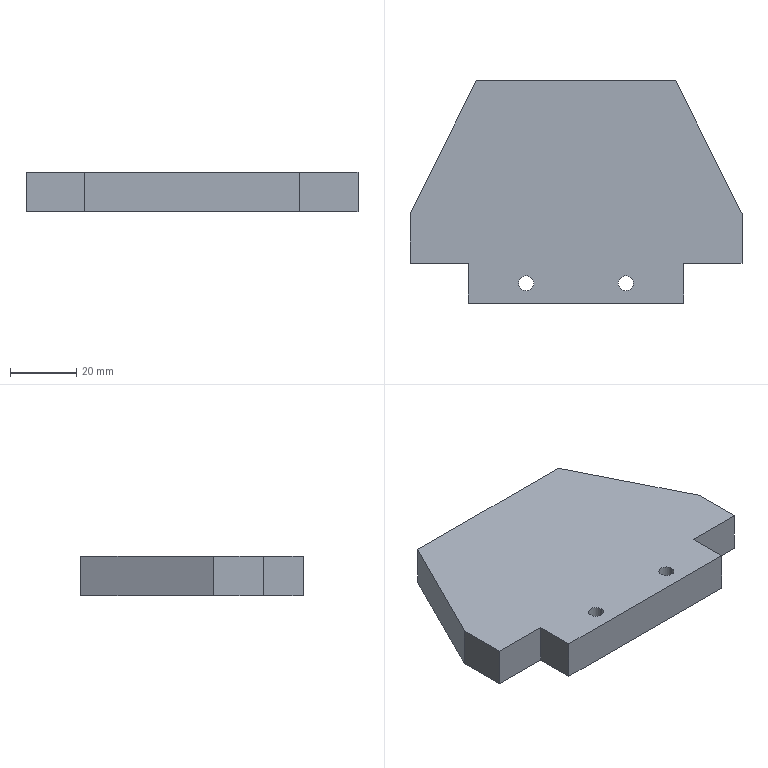Part | SolidWorks | features Chamfer 2, Extrusion 1, HoleWzd 1, ICE 1 | 1 solid | 22 faces | box 100 x 67 x 12 mm | volume 65076 mm3 | plane 14 | cylinder 8 | commonest cylinder face diameters 4.5 x4 8 x4
STEP:
#1=CARTESIAN_POINT('',(-11.,-33.5,4.4));
#2=VERTEX_POINT('',#1);
#3=CARTESIAN_POINT('',(-19.,-33.5,4.4));
#4=VERTEX_POINT('',#3);
#5=CARTESIAN_POINT('',(-15.,-33.5,4.4));
#6=DIRECTION('',(0.,0.,-1.));
#7=DIRECTION('',(-1.,0.,0.));
#8=AXIS2_PLACEMENT_3D('',#5,#6,#7);
#9=CIRCLE('',#8,4.);
#10=EDGE_CURVE('',#2,#4,#9,.T.);
#11=ORIENTED_EDGE('',*,*,#10,.F.);
#12=CARTESIAN_POINT('',(-11.,-33.5,0.));
#13=VERTEX_POINT('',#12);
#14=CARTESIAN_POINT('',(-11.,-33.5,0.));
#15=DIRECTION('',(0.,0.,-1.));
#16=VECTOR('',#15,1000.);
#17=LINE('',#14,#16);
#18=EDGE_CURVE('',#2,#13,#17,.T.);
#19=ORIENTED_EDGE('',*,*,#18,.T.);
#20=CARTESIAN_POINT('',(-19.,-33.5,0.));
#21=VERTEX_POINT('',#20);
#22=CARTESIAN_POINT('',(-15.,-33.5,0.));
#23=DIRECTION('',(0.,0.,-1.));
#24=DIRECTION('',(-1.,0.,0.));
#25=AXIS2_PLACEMENT_3D('',#22,#23,#24);
#26=CIRCLE('',#25,4.);
#27=EDGE_CURVE('',#13,#21,#26,.T.);
#28=ORIENTED_EDGE('',*,*,#27,.T.);
#29=CARTESIAN_POINT('',(-19.,-33.5,0.));
#30=DIRECTION('',(0.,0.,-1.));
#31=VECTOR('',#30,1000.);
#32=LINE('',#29,#31);
#33=EDGE_CURVE('',#4,#21,#32,.T.);
#34=ORIENTED_EDGE('',*,*,#33,.F.);
#35=EDGE_LOOP('',(#11,#19,#28,#34));
#36=FACE_OUTER_BOUND('',#35,.T.);
#37=CARTESIAN_POINT('',(-15.,-33.5,0.));
#38=DIRECTION('',(0.,0.,-1.));
#39=DIRECTION('',(-1.,0.,0.));
#40=AXIS2_PLACEMENT_3D('',#37,#38,#39);
#41=CYLINDRICAL_SURFACE('',#40,4.);
#42=ADVANCED_FACE('',(#36),#41,.F.);
#43=CARTESIAN_POINT('',(-12.75,-33.5,12.));
#44=VERTEX_POINT('',#43);
#45=CARTESIAN_POINT('',(-17.25,-33.5,12.));
#46=VERTEX_POINT('',#45);
#47=CARTESIAN_POINT('',(-15.,-33.5,12.));
#48=DIRECTION('',(0.,0.,-1.));
#49=DIRECTION('',(-1.,0.,0.));
#50=AXIS2_PLACEMENT_3D('',#47,#48,#49);
#51=CIRCLE('',#50,2.25);
#52=EDGE_CURVE('',#44,#46,#51,.T.);
#53=ORIENTED_EDGE('',*,*,#52,.F.);
#54=CARTESIAN_POINT('',(-12.75,-33.5,4.4));
#55=VERTEX_POINT('',#54);
#56=CARTESIAN_POINT('',(-12.75,-33.5,0.));
#57=DIRECTION('',(0.,0.,-1.));
#58=VECTOR('',#57,1000.);
#59=LINE('',#56,#58);
#60=EDGE_CURVE('',#44,#55,#59,.T.);
#61=ORIENTED_EDGE('',*,*,#60,.T.);
#62=CARTESIAN_POINT('',(-17.25,-33.5,4.4));
#63=VERTEX_POINT('',#62);
#64=CARTESIAN_POINT('',(-15.,-33.5,4.4));
#65=DIRECTION('',(0.,0.,-1.));
#66=DIRECTION('',(-1.,0.,0.));
#67=AXIS2_PLACEMENT_3D('',#64,#65,#66);
#68=CIRCLE('',#67,2.25);
#69=EDGE_CURVE('',#55,#63,#68,.T.);
#70=ORIENTED_EDGE('',*,*,#69,.T.);
#71=CARTESIAN_POINT('',(-17.25,-33.5,0.));
#72=DIRECTION('',(0.,0.,-1.));
#73=VECTOR('',#72,1000.);
#74=LINE('',#71,#73);
#75=EDGE_CURVE('',#46,#63,#74,.T.);
#76=ORIENTED_EDGE('',*,*,#75,.F.);
#77=EDGE_LOOP('',(#53,#61,#70,#76));
#78=FACE_OUTER_BOUND('',#77,.T.);
#79=CARTESIAN_POINT('',(-15.,-33.5,0.));
#80=DIRECTION('',(0.,0.,-1.));
#81=DIRECTION('',(-1.,0.,0.));
#82=AXIS2_PLACEMENT_3D('',#79,#80,#81);
#83=CYLINDRICAL_SURFACE('',#82,2.25);
#84=ADVANCED_FACE('',(#78),#83,.F.);
#85=CARTESIAN_POINT('',(19.,-33.5,4.4));
#86=VERTEX_POINT('',#85);
#87=CARTESIAN_POINT('',(11.,-33.5,4.4));
#88=VERTEX_POINT('',#87);
#89=CARTESIAN_POINT('',(15.,-33.5,4.4));
#90=DIRECTION('',(0.,0.,-1.));
#91=DIRECTION('',(-1.,0.,0.));
#92=AXIS2_PLACEMENT_3D('',#89,#90,#91);
#93=CIRCLE('',#92,4.);
#94=EDGE_CURVE('',#86,#88,#93,.T.);
#95=ORIENTED_EDGE('',*,*,#94,.F.);
#96=CARTESIAN_POINT('',(19.,-33.5,0.));
#97=VERTEX_POINT('',#96);
#98=CARTESIAN_POINT('',(19.,-33.5,0.));
#99=DIRECTION('',(0.,0.,-1.));
#100=VECTOR('',#99,1000.);
#101=LINE('',#98,#100);
#102=EDGE_CURVE('',#86,#97,#101,.T.);
#103=ORIENTED_EDGE('',*,*,#102,.T.);
#104=CARTESIAN_POINT('',(11.,-33.5,0.));
#105=VERTEX_POINT('',#104);
#106=CARTESIAN_POINT('',(15.,-33.5,0.));
#107=DIRECTION('',(0.,0.,-1.));
#108=DIRECTION('',(-1.,0.,0.));
#109=AXIS2_PLACEMENT_3D('',#106,#107,#108);
#110=CIRCLE('',#109,4.);
#111=EDGE_CURVE('',#97,#105,#110,.T.);
#112=ORIENTED_EDGE('',*,*,#111,.T.);
#113=CARTESIAN_POINT('',(11.,-33.5,0.));
#114=DIRECTION('',(0.,0.,-1.));
#115=VECTOR('',#114,1000.);
#116=LINE('',#113,#115);
#117=EDGE_CURVE('',#88,#105,#116,.T.);
#118=ORIENTED_EDGE('',*,*,#117,.F.);
#119=EDGE_LOOP('',(#95,#103,#112,#118));
#120=FACE_OUTER_BOUND('',#119,.T.);
#121=CARTESIAN_POINT('',(15.,-33.5,0.));
#122=DIRECTION('',(0.,0.,-1.));
#123=DIRECTION('',(-1.,0.,0.));
#124=AXIS2_PLACEMENT_3D('',#121,#122,#123);
#125=CYLINDRICAL_SURFACE('',#124,4.);
#126=ADVANCED_FACE('',(#120),#125,.F.);
#127=CARTESIAN_POINT('',(17.25,-33.5,12.));
#128=VERTEX_POINT('',#127);
#129=CARTESIAN_POINT('',(12.75,-33.5,12.));
#130=VERTEX_POINT('',#129);
#131=CARTESIAN_POINT('',(15.,-33.5,12.));
#132=DIRECTION('',(0.,0.,-1.));
#133=DIRECTION('',(-1.,0.,0.));
#134=AXIS2_PLACEMENT_3D('',#131,#132,#133);
#135=CIRCLE('',#134,2.25);
#136=EDGE_CURVE('',#128,#130,#135,.T.);
#137=ORIENTED_EDGE('',*,*,#136,.F.);
#138=CARTESIAN_POINT('',(17.25,-33.5,4.4));
#139=VERTEX_POINT('',#138);
#140=CARTESIAN_POINT('',(17.25,-33.5,0.));
#141=DIRECTION('',(0.,0.,-1.));
#142=VECTOR('',#141,1000.);
#143=LINE('',#140,#142);
#144=EDGE_CURVE('',#128,#139,#143,.T.);
#145=ORIENTED_EDGE('',*,*,#144,.T.);
#146=CARTESIAN_POINT('',(12.75,-33.5,4.4));
#147=VERTEX_POINT('',#146);
#148=CARTESIAN_POINT('',(15.,-33.5,4.4));
#149=DIRECTION('',(0.,0.,-1.));
#150=DIRECTION('',(-1.,0.,0.));
#151=AXIS2_PLACEMENT_3D('',#148,#149,#150);
#152=CIRCLE('',#151,2.25);
#153=EDGE_CURVE('',#139,#147,#152,.T.);
#154=ORIENTED_EDGE('',*,*,#153,.T.);
#155=CARTESIAN_POINT('',(12.75,-33.5,0.));
#156=DIRECTION('',(0.,0.,-1.));
#157=VECTOR('',#156,1000.);
#158=LINE('',#155,#157);
#159=EDGE_CURVE('',#130,#147,#158,.T.);
#160=ORIENTED_EDGE('',*,*,#159,.F.);
#161=EDGE_LOOP('',(#137,#145,#154,#160));
#162=FACE_OUTER_BOUND('',#161,.T.);
#163=CARTESIAN_POINT('',(15.,-33.5,0.));
#164=DIRECTION('',(0.,0.,-1.));
#165=DIRECTION('',(-1.,0.,0.));
#166=AXIS2_PLACEMENT_3D('',#163,#164,#165);
#167=CYLINDRICAL_SURFACE('',#166,2.25);
#168=ADVANCED_FACE('',(#162),#167,.F.);
#169=CARTESIAN_POINT('',(-32.5,-27.5,12.));
#170=VERTEX_POINT('',#169);
#171=CARTESIAN_POINT('',(-32.5,-27.5,0.));
#172=VERTEX_POINT('',#171);
#173=CARTESIAN_POINT('',(-32.5,-27.5,12.));
#174=DIRECTION('',(0.,0.,-1.));
#175=VECTOR('',#174,1000.);
#176=LINE('',#173,#175);
#177=EDGE_CURVE('',#170,#172,#176,.T.);
#178=ORIENTED_EDGE('',*,*,#177,.F.);
#179=CARTESIAN_POINT('',(-50.,-27.5,12.));
#180=VERTEX_POINT('',#179);
#181=CARTESIAN_POINT('',(-50.,-27.5,12.));
#182=DIRECTION('',(1.,0.,0.));
#183=VECTOR('',#182,1000.);
#184=LINE('',#181,#183);
#185=EDGE_CURVE('',#180,#170,#184,.T.);
#186=ORIENTED_EDGE('',*,*,#185,.F.);
#187=CARTESIAN_POINT('',(-50.,-27.5,0.));
#188=VERTEX_POINT('',#187);
#189=CARTESIAN_POINT('',(-50.,-27.5,12.));
#190=DIRECTION('',(0.,0.,-1.));
#191=VECTOR('',#190,1000.);
#192=LINE('',#189,#191);
#193=EDGE_CURVE('',#180,#188,#192,.T.);
#194=ORIENTED_EDGE('',*,*,#193,.T.);
#195=CARTESIAN_POINT('',(-50.,-27.5,0.));
#196=DIRECTION('',(1.,0.,0.));
#197=VECTOR('',#196,1000.);
#198=LINE('',#195,#197);
#199=EDGE_CURVE('',#188,#172,#198,.T.);
#200=ORIENTED_EDGE('',*,*,#199,.T.);
#201=EDGE_LOOP('',(#178,#186,#194,#200));
#202=FACE_OUTER_BOUND('',#201,.T.);
#203=CARTESIAN_POINT('',(-50.,-27.5,12.));
#204=DIRECTION('',(0.,1.,0.));
#205=DIRECTION('',(0.,0.,1.));
#206=AXIS2_PLACEMENT_3D('',#203,#204,#205);
#207=PLANE('',#206);
#208=ADVANCED_FACE('',(#202),#207,.F.);
#209=CARTESIAN_POINT('',(32.5,-27.5,0.));
#210=VERTEX_POINT('',#209);
#211=CARTESIAN_POINT('',(32.5,-27.5,12.));
#212=VERTEX_POINT('',#211);
#213=CARTESIAN_POINT('',(32.5,-27.5,12.));
#214=DIRECTION('',(0.,0.,1.));
#215=VECTOR('',#214,1000.);
#216=LINE('',#213,#215);
#217=EDGE_CURVE('',#210,#212,#216,.T.);
#218=ORIENTED_EDGE('',*,*,#217,.F.);
#219=CARTESIAN_POINT('',(50.,-27.5,0.));
#220=VERTEX_POINT('',#219);
#221=CARTESIAN_POINT('',(-50.,-27.5,0.));
#222=DIRECTION('',(1.,0.,0.));
#223=VECTOR('',#222,1000.);
#224=LINE('',#221,#223);
#225=EDGE_CURVE('',#210,#220,#224,.T.);
#226=ORIENTED_EDGE('',*,*,#225,.T.);
#227=CARTESIAN_POINT('',(50.,-27.5,12.));
#228=VERTEX_POINT('',#227);
#229=CARTESIAN_POINT('',(50.,-27.5,12.));
#230=DIRECTION('',(0.,0.,-1.));
#231=VECTOR('',#230,1000.);
#232=LINE('',#229,#231);
#233=EDGE_CURVE('',#228,#220,#232,.T.);
#234=ORIENTED_EDGE('',*,*,#233,.F.);
#235=CARTESIAN_POINT('',(-50.,-27.5,12.));
#236=DIRECTION('',(1.,0.,0.));
#237=VECTOR('',#236,1000.);
#238=LINE('',#235,#237);
#239=EDGE_CURVE('',#212,#228,#238,.T.);
#240=ORIENTED_EDGE('',*,*,#239,.F.);
#241=EDGE_LOOP('',(#218,#226,#234,#240));
#242=FACE_OUTER_BOUND('',#241,.T.);
#243=CARTESIAN_POINT('',(-50.,-27.5,12.));
#244=DIRECTION('',(0.,1.,0.));
#245=DIRECTION('',(0.,0.,1.));
#246=AXIS2_PLACEMENT_3D('',#243,#244,#245);
#247=PLANE('',#246);
#248=ADVANCED_FACE('',(#242),#247,.F.);
#249=CARTESIAN_POINT('',(50.,-12.5,0.));
#250=VERTEX_POINT('',#249);
#251=CARTESIAN_POINT('',(50.,-27.5,0.));
#252=DIRECTION('',(0.,1.,0.));
#253=VECTOR('',#252,1000.);
#254=LINE('',#251,#253);
#255=EDGE_CURVE('',#220,#250,#254,.T.);
#256=ORIENTED_EDGE('',*,*,#255,.T.);
#257=CARTESIAN_POINT('',(50.,-12.5,12.));
#258=VERTEX_POINT('',#257);
#259=CARTESIAN_POINT('',(50.,-12.5,12.));
#260=DIRECTION('',(0.,0.,1.));
#261=VECTOR('',#260,1000.);
#262=LINE('',#259,#261);
#263=EDGE_CURVE('',#250,#258,#262,.T.);
#264=ORIENTED_EDGE('',*,*,#263,.T.);
#265=CARTESIAN_POINT('',(50.,-27.5,12.));
#266=DIRECTION('',(0.,1.,0.));
#267=VECTOR('',#266,1000.);
#268=LINE('',#265,#267);
#269=EDGE_CURVE('',#228,#258,#268,.T.);
#270=ORIENTED_EDGE('',*,*,#269,.F.);
#271=ORIENTED_EDGE('',*,*,#233,.T.);
#272=EDGE_LOOP('',(#256,#264,#270,#271));
#273=FACE_OUTER_BOUND('',#272,.T.);
#274=CARTESIAN_POINT('',(50.,-27.5,12.));
#275=DIRECTION('',(-1.,0.,0.));
#276=DIRECTION('',(0.,0.,1.));
#277=AXIS2_PLACEMENT_3D('',#274,#275,#276);
#278=PLANE('',#277);
#279=ADVANCED_FACE('',(#273),#278,.F.);
#280=CARTESIAN_POINT('',(30.,27.5,0.));
#281=VERTEX_POINT('',#280);
#282=CARTESIAN_POINT('',(-30.,27.5,0.));
#283=VERTEX_POINT('',#282);
#284=CARTESIAN_POINT('',(-50.,27.5,0.));
#285=DIRECTION('',(-1.,0.,0.));
#286=VECTOR('',#285,1000.);
#287=LINE('',#284,#286);
#288=EDGE_CURVE('',#281,#283,#287,.T.);
#289=ORIENTED_EDGE('',*,*,#288,.T.);
#290=CARTESIAN_POINT('',(-30.,27.5,12.));
#291=VERTEX_POINT('',#290);
#292=CARTESIAN_POINT('',(-30.,27.5,12.));
#293=DIRECTION('',(0.,0.,1.));
#294=VECTOR('',#293,1000.);
#295=LINE('',#292,#294);
#296=EDGE_CURVE('',#283,#291,#295,.T.);
#297=ORIENTED_EDGE('',*,*,#296,.T.);
#298=CARTESIAN_POINT('',(30.,27.5,12.));
#299=VERTEX_POINT('',#298);
#300=CARTESIAN_POINT('',(-50.,27.5,12.));
#301=DIRECTION('',(-1.,0.,0.));
#302=VECTOR('',#301,1000.);
#303=LINE('',#300,#302);
#304=EDGE_CURVE('',#299,#291,#303,.T.);
#305=ORIENTED_EDGE('',*,*,#304,.F.);
#306=CARTESIAN_POINT('',(30.,27.5,12.));
#307=DIRECTION('',(0.,0.,-1.));
#308=VECTOR('',#307,1000.);
#309=LINE('',#306,#308);
#310=EDGE_CURVE('',#299,#281,#309,.T.);
#311=ORIENTED_EDGE('',*,*,#310,.T.);
#312=EDGE_LOOP('',(#289,#297,#305,#311));
#313=FACE_OUTER_BOUND('',#312,.T.);
#314=CARTESIAN_POINT('',(-50.,27.5,12.));
#315=DIRECTION('',(0.,-1.,0.));
#316=DIRECTION('',(0.,0.,-1.));
#317=AXIS2_PLACEMENT_3D('',#314,#315,#316);
#318=PLANE('',#317);
#319=ADVANCED_FACE('',(#313),#318,.F.);
#320=CARTESIAN_POINT('',(-50.,-12.5,12.));
#321=VERTEX_POINT('',#320);
#322=CARTESIAN_POINT('',(-50.,-27.5,12.));
#323=DIRECTION('',(0.,-1.,0.));
#324=VECTOR('',#323,1000.);
#325=LINE('',#322,#324);
#326=EDGE_CURVE('',#321,#180,#325,.T.);
#327=ORIENTED_EDGE('',*,*,#326,.F.);
#328=CARTESIAN_POINT('',(-50.,-12.5,0.));
#329=VERTEX_POINT('',#328);
#330=CARTESIAN_POINT('',(-50.,-12.5,12.));
#331=DIRECTION('',(0.,0.,-1.));
#332=VECTOR('',#331,1000.);
#333=LINE('',#330,#332);
#334=EDGE_CURVE('',#321,#329,#333,.T.);
#335=ORIENTED_EDGE('',*,*,#334,.T.);
#336=CARTESIAN_POINT('',(-50.,-27.5,0.));
#337=DIRECTION('',(0.,-1.,0.));
#338=VECTOR('',#337,1000.);
#339=LINE('',#336,#338);
#340=EDGE_CURVE('',#329,#188,#339,.T.);
#341=ORIENTED_EDGE('',*,*,#340,.T.);
#342=ORIENTED_EDGE('',*,*,#193,.F.);
#343=EDGE_LOOP('',(#327,#335,#341,#342));
#344=FACE_OUTER_BOUND('',#343,.T.);
#345=CARTESIAN_POINT('',(-50.,-27.5,12.));
#346=DIRECTION('',(1.,0.,0.));
#347=DIRECTION('',(0.,0.,-1.));
#348=AXIS2_PLACEMENT_3D('',#345,#346,#347);
#349=PLANE('',#348);
#350=ADVANCED_FACE('',(#344),#349,.F.);
#351=CARTESIAN_POINT('',(-15.,-33.5,12.));
#352=DIRECTION('',(0.,0.,-1.));
#353=DIRECTION('',(-1.,0.,0.));
#354=AXIS2_PLACEMENT_3D('',#351,#352,#353);
#355=CIRCLE('',#354,2.25);
#356=EDGE_CURVE('',#46,#44,#355,.T.);
#357=ORIENTED_EDGE('',*,*,#356,.T.);
#358=ORIENTED_EDGE('',*,*,#52,.T.);
#359=EDGE_LOOP('',(#357,#358));
#360=FACE_BOUND('',#359,.T.);
#361=CARTESIAN_POINT('',(15.,-33.5,12.));
#362=DIRECTION('',(0.,0.,-1.));
#363=DIRECTION('',(-1.,0.,0.));
#364=AXIS2_PLACEMENT_3D('',#361,#362,#363);
#365=CIRCLE('',#364,2.25);
#366=EDGE_CURVE('',#130,#128,#365,.T.);
#367=ORIENTED_EDGE('',*,*,#366,.T.);
#368=ORIENTED_EDGE('',*,*,#136,.T.);
#369=EDGE_LOOP('',(#367,#368));
#370=FACE_BOUND('',#369,.T.);
#371=ORIENTED_EDGE('',*,*,#304,.T.);
#372=CARTESIAN_POINT('',(-50.,-12.5,12.));
#373=DIRECTION('',(-0.4472,-0.8944,0.));
#374=VECTOR('',#373,1000.);
#375=LINE('',#372,#374);
#376=EDGE_CURVE('',#291,#321,#375,.T.);
#377=ORIENTED_EDGE('',*,*,#376,.T.);
#378=ORIENTED_EDGE('',*,*,#326,.T.);
#379=ORIENTED_EDGE('',*,*,#185,.T.);
#380=CARTESIAN_POINT('',(-32.5,-39.5,12.));
#381=VERTEX_POINT('',#380);
#382=CARTESIAN_POINT('',(-32.5,-39.5,12.));
#383=DIRECTION('',(0.,1.,0.));
#384=VECTOR('',#383,1000.);
#385=LINE('',#382,#384);
#386=EDGE_CURVE('',#381,#170,#385,.T.);
#387=ORIENTED_EDGE('',*,*,#386,.F.);
#388=CARTESIAN_POINT('',(32.5,-39.5,12.));
#389=VERTEX_POINT('',#388);
#390=CARTESIAN_POINT('',(-32.5,-39.5,12.));
#391=DIRECTION('',(-1.,0.,0.));
#392=VECTOR('',#391,1000.);
#393=LINE('',#390,#392);
#394=EDGE_CURVE('',#389,#381,#393,.T.);
#395=ORIENTED_EDGE('',*,*,#394,.F.);
#396=CARTESIAN_POINT('',(32.5,-39.5,12.));
#397=DIRECTION('',(0.,1.,0.));
#398=VECTOR('',#397,1000.);
#399=LINE('',#396,#398);
#400=EDGE_CURVE('',#389,#212,#399,.T.);
#401=ORIENTED_EDGE('',*,*,#400,.T.);
#402=ORIENTED_EDGE('',*,*,#239,.T.);
#403=ORIENTED_EDGE('',*,*,#269,.T.);
#404=CARTESIAN_POINT('',(30.,27.5,12.));
#405=DIRECTION('',(-0.4472,0.8944,0.));
#406=VECTOR('',#405,1000.);
#407=LINE('',#404,#406);
#408=EDGE_CURVE('',#258,#299,#407,.T.);
#409=ORIENTED_EDGE('',*,*,#408,.T.);
#410=EDGE_LOOP('',(#371,#377,#378,#379,#387,#395,#401,#402,#403,#409));
#411=FACE_OUTER_BOUND('',#410,.T.);
#412=CARTESIAN_POINT('',(0.,0.,12.));
#413=DIRECTION('',(0.,0.,-1.));
#414=DIRECTION('',(-1.,0.,0.));
#415=AXIS2_PLACEMENT_3D('',#412,#413,#414);
#416=PLANE('',#415);
#417=ADVANCED_FACE('',(#360,#370,#411),#416,.F.);
#418=CARTESIAN_POINT('',(-15.,-33.5,0.));
#419=DIRECTION('',(0.,0.,-1.));
#420=DIRECTION('',(-1.,0.,0.));
#421=AXIS2_PLACEMENT_3D('',#418,#419,#420);
#422=CIRCLE('',#421,4.);
#423=EDGE_CURVE('',#21,#13,#422,.T.);
#424=ORIENTED_EDGE('',*,*,#423,.F.);
#425=ORIENTED_EDGE('',*,*,#27,.F.);
#426=EDGE_LOOP('',(#424,#425));
#427=FACE_BOUND('',#426,.T.);
#428=CARTESIAN_POINT('',(15.,-33.5,0.));
#429=DIRECTION('',(0.,0.,-1.));
#430=DIRECTION('',(-1.,0.,0.));
#431=AXIS2_PLACEMENT_3D('',#428,#429,#430);
#432=CIRCLE('',#431,4.);
#433=EDGE_CURVE('',#105,#97,#432,.T.);
#434=ORIENTED_EDGE('',*,*,#433,.F.);
#435=ORIENTED_EDGE('',*,*,#111,.F.);
#436=EDGE_LOOP('',(#434,#435));
#437=FACE_BOUND('',#436,.T.);
#438=ORIENTED_EDGE('',*,*,#340,.F.);
#439=CARTESIAN_POINT('',(-35.,17.5,0.));
#440=DIRECTION('',(0.4472,0.8944,0.));
#441=VECTOR('',#440,1000.);
#442=LINE('',#439,#441);
#443=EDGE_CURVE('',#329,#283,#442,.T.);
#444=ORIENTED_EDGE('',*,*,#443,.T.);
#445=ORIENTED_EDGE('',*,*,#288,.F.);
#446=CARTESIAN_POINT('',(35.,17.5,0.));
#447=DIRECTION('',(0.4472,-0.8944,0.));
#448=VECTOR('',#447,1000.);
#449=LINE('',#446,#448);
#450=EDGE_CURVE('',#281,#250,#449,.T.);
#451=ORIENTED_EDGE('',*,*,#450,.T.);
#452=ORIENTED_EDGE('',*,*,#255,.F.);
#453=ORIENTED_EDGE('',*,*,#225,.F.);
#454=CARTESIAN_POINT('',(32.5,-39.5,0.));
#455=VERTEX_POINT('',#454);
#456=CARTESIAN_POINT('',(32.5,-39.5,0.));
#457=DIRECTION('',(0.,1.,0.));
#458=VECTOR('',#457,1000.);
#459=LINE('',#456,#458);
#460=EDGE_CURVE('',#455,#210,#459,.T.);
#461=ORIENTED_EDGE('',*,*,#460,.F.);
#462=CARTESIAN_POINT('',(-32.5,-39.5,0.));
#463=VERTEX_POINT('',#462);
#464=CARTESIAN_POINT('',(-32.5,-39.5,0.));
#465=DIRECTION('',(1.,0.,0.));
#466=VECTOR('',#465,1000.);
#467=LINE('',#464,#466);
#468=EDGE_CURVE('',#463,#455,#467,.T.);
#469=ORIENTED_EDGE('',*,*,#468,.F.);
#470=CARTESIAN_POINT('',(-32.5,-39.5,0.));
#471=DIRECTION('',(0.,1.,0.));
#472=VECTOR('',#471,1000.);
#473=LINE('',#470,#472);
#474=EDGE_CURVE('',#463,#172,#473,.T.);
#475=ORIENTED_EDGE('',*,*,#474,.T.);
#476=ORIENTED_EDGE('',*,*,#199,.F.);
#477=EDGE_LOOP('',(#438,#444,#445,#451,#452,#453,#461,#469,#475,#476));
#478=FACE_OUTER_BOUND('',#477,.T.);
#479=CARTESIAN_POINT('',(0.,0.,0.));
#480=DIRECTION('',(0.,0.,-1.));
#481=DIRECTION('',(-1.,0.,0.));
#482=AXIS2_PLACEMENT_3D('',#479,#480,#481);
#483=PLANE('',#482);
#484=ADVANCED_FACE('',(#427,#437,#478),#483,.T.);
#485=ORIENTED_EDGE('',*,*,#177,.T.);
#486=ORIENTED_EDGE('',*,*,#474,.F.);
#487=CARTESIAN_POINT('',(-32.5,-39.5,12.));
#488=DIRECTION('',(0.,0.,-1.));
#489=VECTOR('',#488,1000.);
#490=LINE('',#487,#489);
#491=EDGE_CURVE('',#381,#463,#490,.T.);
#492=ORIENTED_EDGE('',*,*,#491,.F.);
#493=ORIENTED_EDGE('',*,*,#386,.T.);
#494=EDGE_LOOP('',(#485,#486,#492,#493));
#495=FACE_OUTER_BOUND('',#494,.T.);
#496=CARTESIAN_POINT('',(-32.5,-39.5,12.));
#497=DIRECTION('',(1.,0.,0.));
#498=DIRECTION('',(0.,0.,-1.));
#499=AXIS2_PLACEMENT_3D('',#496,#497,#498);
#500=PLANE('',#499);
#501=ADVANCED_FACE('',(#495),#500,.F.);
#502=ORIENTED_EDGE('',*,*,#217,.T.);
#503=ORIENTED_EDGE('',*,*,#400,.F.);
#504=CARTESIAN_POINT('',(32.5,-39.5,12.));
#505=DIRECTION('',(0.,0.,1.));
#506=VECTOR('',#505,1000.);
#507=LINE('',#504,#506);
#508=EDGE_CURVE('',#455,#389,#507,.T.);
#509=ORIENTED_EDGE('',*,*,#508,.F.);
#510=ORIENTED_EDGE('',*,*,#460,.T.);
#511=EDGE_LOOP('',(#502,#503,#509,#510));
#512=FACE_OUTER_BOUND('',#511,.T.);
#513=CARTESIAN_POINT('',(32.5,-39.5,12.));
#514=DIRECTION('',(-1.,0.,0.));
#515=DIRECTION('',(0.,0.,1.));
#516=AXIS2_PLACEMENT_3D('',#513,#514,#515);
#517=PLANE('',#516);
#518=ADVANCED_FACE('',(#512),#517,.F.);
#519=ORIENTED_EDGE('',*,*,#491,.T.);
#520=ORIENTED_EDGE('',*,*,#468,.T.);
#521=ORIENTED_EDGE('',*,*,#508,.T.);
#522=ORIENTED_EDGE('',*,*,#394,.T.);
#523=EDGE_LOOP('',(#519,#520,#521,#522));
#524=FACE_OUTER_BOUND('',#523,.T.);
#525=CARTESIAN_POINT('',(0.,-39.5,0.));
#526=DIRECTION('',(0.,-1.,0.));
#527=DIRECTION('',(0.,0.,-1.));
#528=AXIS2_PLACEMENT_3D('',#525,#526,#527);
#529=PLANE('',#528);
#530=ADVANCED_FACE('',(#524),#529,.T.);
#531=ORIENTED_EDGE('',*,*,#144,.F.);
#532=ORIENTED_EDGE('',*,*,#366,.F.);
#533=ORIENTED_EDGE('',*,*,#159,.T.);
#534=CARTESIAN_POINT('',(15.,-33.5,4.4));
#535=DIRECTION('',(0.,0.,-1.));
#536=DIRECTION('',(-1.,0.,0.));
#537=AXIS2_PLACEMENT_3D('',#534,#535,#536);
#538=CIRCLE('',#537,2.25);
#539=EDGE_CURVE('',#147,#139,#538,.T.);
#540=ORIENTED_EDGE('',*,*,#539,.T.);
#541=EDGE_LOOP('',(#531,#532,#533,#540));
#542=FACE_OUTER_BOUND('',#541,.T.);
#543=CARTESIAN_POINT('',(15.,-33.5,0.));
#544=DIRECTION('',(0.,0.,-1.));
#545=DIRECTION('',(-1.,0.,0.));
#546=AXIS2_PLACEMENT_3D('',#543,#544,#545);
#547=CYLINDRICAL_SURFACE('',#546,2.25);
#548=ADVANCED_FACE('',(#542),#547,.F.);
#549=ORIENTED_EDGE('',*,*,#539,.F.);
#550=ORIENTED_EDGE('',*,*,#153,.F.);
#551=EDGE_LOOP('',(#549,#550));
#552=FACE_BOUND('',#551,.T.);
#553=CARTESIAN_POINT('',(15.,-33.5,4.4));
#554=DIRECTION('',(0.,0.,-1.));
#555=DIRECTION('',(-1.,0.,0.));
#556=AXIS2_PLACEMENT_3D('',#553,#554,#555);
#557=CIRCLE('',#556,4.);
#558=EDGE_CURVE('',#88,#86,#557,.T.);
#559=ORIENTED_EDGE('',*,*,#558,.T.);
#560=ORIENTED_EDGE('',*,*,#94,.T.);
#561=EDGE_LOOP('',(#559,#560));
#562=FACE_OUTER_BOUND('',#561,.T.);
#563=CARTESIAN_POINT('',(17.25,-33.5,4.4));
#564=DIRECTION('',(0.,0.,1.));
#565=DIRECTION('',(1.,0.,0.));
#566=AXIS2_PLACEMENT_3D('',#563,#564,#565);
#567=PLANE('',#566);
#568=ADVANCED_FACE('',(#552,#562),#567,.F.);
#569=ORIENTED_EDGE('',*,*,#102,.F.);
#570=ORIENTED_EDGE('',*,*,#558,.F.);
#571=ORIENTED_EDGE('',*,*,#117,.T.);
#572=ORIENTED_EDGE('',*,*,#433,.T.);
#573=EDGE_LOOP('',(#569,#570,#571,#572));
#574=FACE_OUTER_BOUND('',#573,.T.);
#575=CARTESIAN_POINT('',(15.,-33.5,0.));
#576=DIRECTION('',(0.,0.,-1.));
#577=DIRECTION('',(-1.,0.,0.));
#578=AXIS2_PLACEMENT_3D('',#575,#576,#577);
#579=CYLINDRICAL_SURFACE('',#578,4.);
#580=ADVANCED_FACE('',(#574),#579,.F.);
#581=ORIENTED_EDGE('',*,*,#60,.F.);
#582=ORIENTED_EDGE('',*,*,#356,.F.);
#583=ORIENTED_EDGE('',*,*,#75,.T.);
#584=CARTESIAN_POINT('',(-15.,-33.5,4.4));
#585=DIRECTION('',(0.,0.,-1.));
#586=DIRECTION('',(-1.,0.,0.));
#587=AXIS2_PLACEMENT_3D('',#584,#585,#586);
#588=CIRCLE('',#587,2.25);
#589=EDGE_CURVE('',#63,#55,#588,.T.);
#590=ORIENTED_EDGE('',*,*,#589,.T.);
#591=EDGE_LOOP('',(#581,#582,#583,#590));
#592=FACE_OUTER_BOUND('',#591,.T.);
#593=CARTESIAN_POINT('',(-15.,-33.5,0.));
#594=DIRECTION('',(0.,0.,-1.));
#595=DIRECTION('',(-1.,0.,0.));
#596=AXIS2_PLACEMENT_3D('',#593,#594,#595);
#597=CYLINDRICAL_SURFACE('',#596,2.25);
#598=ADVANCED_FACE('',(#592),#597,.F.);
#599=ORIENTED_EDGE('',*,*,#589,.F.);
#600=ORIENTED_EDGE('',*,*,#69,.F.);
#601=EDGE_LOOP('',(#599,#600));
#602=FACE_BOUND('',#601,.T.);
#603=CARTESIAN_POINT('',(-15.,-33.5,4.4));
#604=DIRECTION('',(0.,0.,-1.));
#605=DIRECTION('',(-1.,0.,0.));
#606=AXIS2_PLACEMENT_3D('',#603,#604,#605);
#607=CIRCLE('',#606,4.);
#608=EDGE_CURVE('',#4,#2,#607,.T.);
#609=ORIENTED_EDGE('',*,*,#608,.T.);
#610=ORIENTED_EDGE('',*,*,#10,.T.);
#611=EDGE_LOOP('',(#609,#610));
#612=FACE_OUTER_BOUND('',#611,.T.);
#613=CARTESIAN_POINT('',(-12.75,-33.5,4.4));
#614=DIRECTION('',(0.,0.,1.));
#615=DIRECTION('',(1.,0.,0.));
#616=AXIS2_PLACEMENT_3D('',#613,#614,#615);
#617=PLANE('',#616);
#618=ADVANCED_FACE('',(#602,#612),#617,.F.);
#619=ORIENTED_EDGE('',*,*,#18,.F.);
#620=ORIENTED_EDGE('',*,*,#608,.F.);
#621=ORIENTED_EDGE('',*,*,#33,.T.);
#622=ORIENTED_EDGE('',*,*,#423,.T.);
#623=EDGE_LOOP('',(#619,#620,#621,#622));
#624=FACE_OUTER_BOUND('',#623,.T.);
#625=CARTESIAN_POINT('',(-15.,-33.5,0.));
#626=DIRECTION('',(0.,0.,-1.));
#627=DIRECTION('',(-1.,0.,0.));
#628=AXIS2_PLACEMENT_3D('',#625,#626,#627);
#629=CYLINDRICAL_SURFACE('',#628,4.);
#630=ADVANCED_FACE('',(#624),#629,.F.);
#631=ORIENTED_EDGE('',*,*,#408,.F.);
#632=ORIENTED_EDGE('',*,*,#263,.F.);
#633=ORIENTED_EDGE('',*,*,#450,.F.);
#634=ORIENTED_EDGE('',*,*,#310,.F.);
#635=EDGE_LOOP('',(#631,#632,#633,#634));
#636=FACE_OUTER_BOUND('',#635,.T.);
#637=CARTESIAN_POINT('',(30.,27.5,12.));
#638=DIRECTION('',(-0.8944,-0.4472,0.));
#639=DIRECTION('',(0.,0.,-1.));
#640=AXIS2_PLACEMENT_3D('',#637,#638,#639);
#641=PLANE('',#640);
#642=ADVANCED_FACE('',(#636),#641,.F.);
#643=ORIENTED_EDGE('',*,*,#376,.F.);
#644=ORIENTED_EDGE('',*,*,#296,.F.);
#645=ORIENTED_EDGE('',*,*,#443,.F.);
#646=ORIENTED_EDGE('',*,*,#334,.F.);
#647=EDGE_LOOP('',(#643,#644,#645,#646));
#648=FACE_OUTER_BOUND('',#647,.T.);
#649=CARTESIAN_POINT('',(-50.,-12.5,12.));
#650=DIRECTION('',(0.8944,-0.4472,0.));
#651=DIRECTION('',(0.,0.,-1.));
#652=AXIS2_PLACEMENT_3D('',#649,#650,#651);
#653=PLANE('',#652);
#654=ADVANCED_FACE('',(#648),#653,.F.);
#655=CLOSED_SHELL('',(#42,#84,#126,#168,#208,#248,#279,#319,#350,#417,#484,#501,#518,#530,#548,#568,#580,#598,#618,#630,#642,#654));
#656=MANIFOLD_SOLID_BREP('',#655);
#657=CARTESIAN_POINT('',(0.,0.,0.));
#658=DIRECTION('',(0.,0.,1.));
#659=DIRECTION('',(1.,0.,0.));
#660=AXIS2_PLACEMENT_3D('',#657,#658,#659);
#661=(LENGTH_UNIT()NAMED_UNIT(*)SI_UNIT(.MILLI.,.METRE.));
#662=UNCERTAINTY_MEASURE_WITH_UNIT(LENGTH_MEASURE(0.00001),#661,'','');
#663=(NAMED_UNIT(*)PLANE_ANGLE_UNIT()SI_UNIT($,.RADIAN.));
#664=(NAMED_UNIT(*)SI_UNIT($,.STERADIAN.)SOLID_ANGLE_UNIT());
#665=(GEOMETRIC_REPRESENTATION_CONTEXT(3)GLOBAL_UNCERTAINTY_ASSIGNED_CONTEXT((#662))GLOBAL_UNIT_ASSIGNED_CONTEXT((#661,#663,#664))REPRESENTATION_CONTEXT('',''));
#666=ADVANCED_BREP_SHAPE_REPRESENTATION('',(#656,#660),#665);